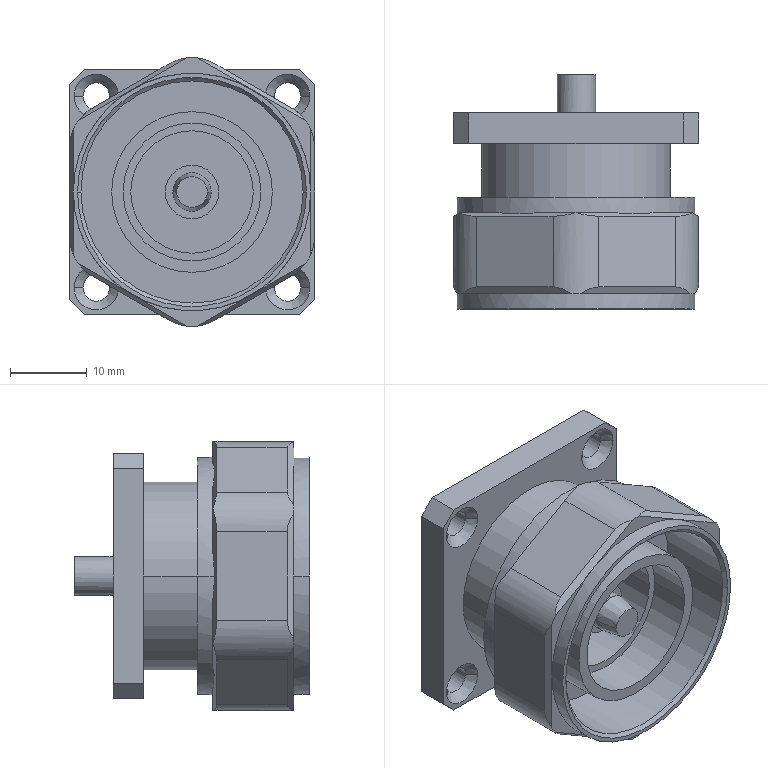Part | STEP file | Connector L29-JFD | 4 solids | 116 faces | box 32 x 30.6 x 35.094 mm | volume 12630 mm3 | plane 58 | cylinder 44 | cone 14 | commonest cylinder face diameters 3.5 x8 5 x7 12 x6 16 x5 24.6 x4 29 x4